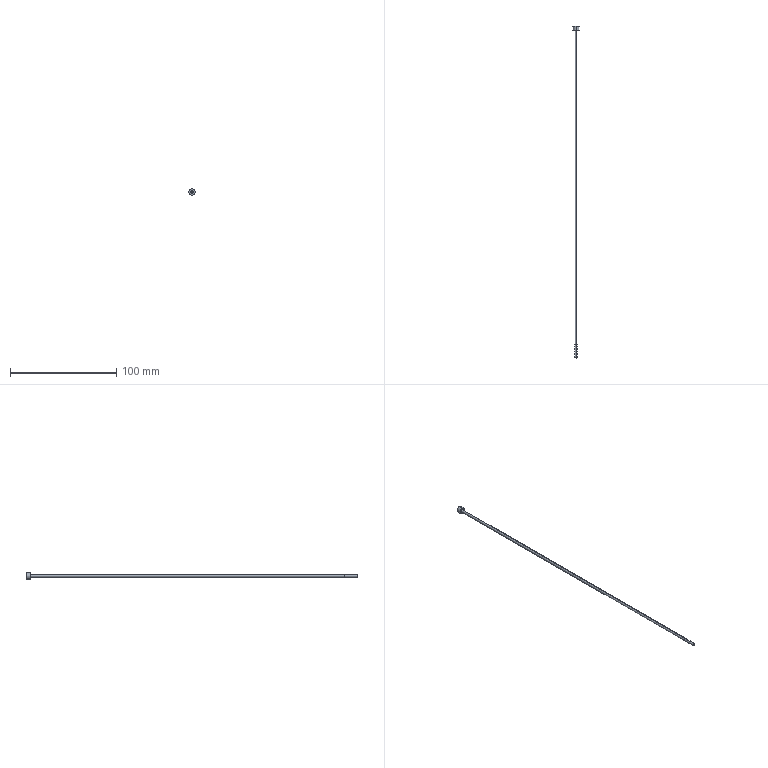Part | STEP file | 1 solid | 9 faces | box 6 x 312.335 x 6 mm | volume 1622 mm3 | cylinder 4 | plane 3 | cone 2 | commonest cylinder face diameters 2.5 x2 6 x2
STEP:
#1=CARTESIAN_POINT('',(0.,0.,0.));
#2=DIRECTION('',(0.,0.,1.));
#3=DIRECTION('',(1.,0.,0.));
#4=AXIS2_PLACEMENT_3D('',#1,#2,#3);
#5=CARTESIAN_POINT('',(-108.037,345.5,10.065));
#6=VERTEX_POINT('',#5);
#7=CARTESIAN_POINT('',(-108.037,345.5,16.065));
#8=VERTEX_POINT('',#7);
#9=CARTESIAN_POINT('',(-108.037,345.5,13.065));
#10=DIRECTION('',(0.,-1.,0.));
#11=DIRECTION('',(0.,0.,-1.));
#12=AXIS2_PLACEMENT_3D('',#9,#10,#11);
#13=CIRCLE('',#12,3.);
#14=CARTESIAN_POINT('',(-108.037,345.5,13.065));
#15=DIRECTION('',(0.,-1.,0.));
#16=DIRECTION('',(0.,0.,-1.));
#17=AXIS2_PLACEMENT_3D('',#14,#15,#16);
#18=CYLINDRICAL_SURFACE('',#17,3.);
#19=CARTESIAN_POINT('',(0.,0.));
#20=DIRECTION('',(1.,0.));
#21=VECTOR('',#20,1.);
#22=LINE('',#19,#21);
#23=(GEOMETRIC_REPRESENTATION_CONTEXT(2)PARAMETRIC_REPRESENTATION_CONTEXT()REPRESENTATION_CONTEXT('',''));
#24=DEFINITIONAL_REPRESENTATION('',(#22),#23);
#25=PCURVE('',#18,#24);
#26=CARTESIAN_POINT('',(-72.862,345.5,110.196));
#27=DIRECTION('',(0.,-1.,0.));
#28=DIRECTION('',(0.,0.,-1.));
#29=AXIS2_PLACEMENT_3D('',#26,#27,#28);
#30=PLANE('',#29);
#31=CARTESIAN_POINT('',(97.131,-35.175));
#32=DIRECTION('',(1.,0.));
#33=AXIS2_PLACEMENT_2D('',#31,#32);
#34=CIRCLE('',#33,3.);
#35=(GEOMETRIC_REPRESENTATION_CONTEXT(2)PARAMETRIC_REPRESENTATION_CONTEXT()REPRESENTATION_CONTEXT('',''));
#36=DEFINITIONAL_REPRESENTATION('',(#34),#35);
#37=PCURVE('',#30,#36);
#38=SURFACE_CURVE('',#13,(#25,#37),.PCURVE_S1.);
#39=EDGE_CURVE('',#6,#8,#38,.T.);
#40=ORIENTED_EDGE('',*,*,#39,.T.);
#41=CARTESIAN_POINT('',(-108.037,341.5,16.065));
#42=VERTEX_POINT('',#41);
#43=CARTESIAN_POINT('',(-108.037,345.5,16.065));
#44=DIRECTION('',(0.,-1.,0.));
#45=VECTOR('',#44,1.);
#46=LINE('',#43,#45);
#47=CARTESIAN_POINT('',(3.142,0.));
#48=DIRECTION('',(0.,1.));
#49=VECTOR('',#48,1.);
#50=LINE('',#47,#49);
#51=(GEOMETRIC_REPRESENTATION_CONTEXT(2)PARAMETRIC_REPRESENTATION_CONTEXT()REPRESENTATION_CONTEXT('',''));
#52=DEFINITIONAL_REPRESENTATION('',(#50),#51);
#53=PCURVE('',#18,#52);
#54=CARTESIAN_POINT('',(-108.037,345.5,13.065));
#55=DIRECTION('',(0.,-1.,0.));
#56=DIRECTION('',(0.,0.,-1.));
#57=AXIS2_PLACEMENT_3D('',#54,#55,#56);
#58=CYLINDRICAL_SURFACE('',#57,3.);
#59=CARTESIAN_POINT('',(3.142,0.));
#60=DIRECTION('',(0.,1.));
#61=VECTOR('',#60,1.);
#62=LINE('',#59,#61);
#63=(GEOMETRIC_REPRESENTATION_CONTEXT(2)PARAMETRIC_REPRESENTATION_CONTEXT()REPRESENTATION_CONTEXT('',''));
#64=DEFINITIONAL_REPRESENTATION('',(#62),#63);
#65=PCURVE('',#58,#64);
#66=SURFACE_CURVE('',#46,(#53,#65),.PCURVE_S1.);
#67=EDGE_CURVE('',#8,#42,#66,.T.);
#68=ORIENTED_EDGE('',*,*,#67,.T.);
#69=CARTESIAN_POINT('',(-108.037,341.5,10.065));
#70=VERTEX_POINT('',#69);
#71=CARTESIAN_POINT('',(-108.037,341.5,13.065));
#72=DIRECTION('',(0.,1.,0.));
#73=DIRECTION('',(0.,0.,1.));
#74=AXIS2_PLACEMENT_3D('',#71,#72,#73);
#75=CIRCLE('',#74,3.);
#76=CARTESIAN_POINT('',(3.142,4.));
#77=DIRECTION('',(-1.,0.));
#78=VECTOR('',#77,1.);
#79=LINE('',#76,#78);
#80=(GEOMETRIC_REPRESENTATION_CONTEXT(2)PARAMETRIC_REPRESENTATION_CONTEXT()REPRESENTATION_CONTEXT('',''));
#81=DEFINITIONAL_REPRESENTATION('',(#79),#80);
#82=PCURVE('',#18,#81);
#83=CARTESIAN_POINT('',(-108.037,341.5,13.065));
#84=DIRECTION('',(0.,-1.,0.));
#85=DIRECTION('',(0.,0.,-1.));
#86=AXIS2_PLACEMENT_3D('',#83,#84,#85);
#87=PLANE('',#86);
#88=CARTESIAN_POINT('',(-3.,0.));
#89=CARTESIAN_POINT('',(-3.,5.196));
#90=CARTESIAN_POINT('',(1.5,2.598));
#91=CARTESIAN_POINT('',(6.,0.));
#92=CARTESIAN_POINT('',(1.5,-2.598));
#93=CARTESIAN_POINT('',(-3.,-5.196));
#94=CARTESIAN_POINT('',(-3.,0.));
#95=(BOUNDED_CURVE()B_SPLINE_CURVE(2,(#88,#89,#90,#91,#92,#93,#94),.UNSPECIFIED.,.T.,.F.)B_SPLINE_CURVE_WITH_KNOTS((1,2,2,2,2,1),(-2.094,0.,2.094,4.189,6.283,8.378),.UNSPECIFIED.)CURVE()GEOMETRIC_REPRESENTATION_ITEM()RATIONAL_B_SPLINE_CURVE((1.,0.5,1.,0.5,1.,0.5,1.))REPRESENTATION_ITEM(''));
#96=(GEOMETRIC_REPRESENTATION_CONTEXT(2)PARAMETRIC_REPRESENTATION_CONTEXT()REPRESENTATION_CONTEXT('',''));
#97=DEFINITIONAL_REPRESENTATION('',(#95),#96);
#98=PCURVE('',#87,#97);
#99=SURFACE_CURVE('',#75,(#82,#98),.PCURVE_S1.);
#100=EDGE_CURVE('',#42,#70,#99,.T.);
#101=ORIENTED_EDGE('',*,*,#100,.T.);
#102=CARTESIAN_POINT('',(-108.037,345.5,10.065));
#103=DIRECTION('',(0.,-1.,0.));
#104=VECTOR('',#103,1.);
#105=LINE('',#102,#104);
#106=CARTESIAN_POINT('',(0.,0.));
#107=DIRECTION('',(0.,1.));
#108=VECTOR('',#107,1.);
#109=LINE('',#106,#108);
#110=(GEOMETRIC_REPRESENTATION_CONTEXT(2)PARAMETRIC_REPRESENTATION_CONTEXT()REPRESENTATION_CONTEXT('',''));
#111=DEFINITIONAL_REPRESENTATION('',(#109),#110);
#112=PCURVE('',#18,#111);
#113=CARTESIAN_POINT('',(6.283,0.));
#114=DIRECTION('',(0.,1.));
#115=VECTOR('',#114,1.);
#116=LINE('',#113,#115);
#117=(GEOMETRIC_REPRESENTATION_CONTEXT(2)PARAMETRIC_REPRESENTATION_CONTEXT()REPRESENTATION_CONTEXT('',''));
#118=DEFINITIONAL_REPRESENTATION('',(#116),#117);
#119=PCURVE('',#58,#118);
#120=SURFACE_CURVE('',#105,(#112,#119),.PCURVE_S1.);
#121=EDGE_CURVE('',#6,#70,#120,.T.);
#122=ORIENTED_EDGE('',*,*,#121,.F.);
#123=EDGE_LOOP('',(#40,#68,#101,#122));
#124=FACE_BOUND('',#123,.T.);
#125=ADVANCED_FACE('',(#124),#18,.T.);
#126=CARTESIAN_POINT('',(-108.037,33.165,14.207));
#127=VERTEX_POINT('',#126);
#128=CARTESIAN_POINT('',(-108.037,33.165,11.923));
#129=VERTEX_POINT('',#128);
#130=CARTESIAN_POINT('',(-108.037,33.165,13.065));
#131=DIRECTION('',(0.,1.,0.));
#132=DIRECTION('',(0.,0.,-1.));
#133=AXIS2_PLACEMENT_3D('',#130,#131,#132);
#134=CIRCLE('',#133,1.142);
#135=CARTESIAN_POINT('',(-108.037,46.23,13.065));
#136=DIRECTION('',(0.,1.,0.));
#137=DIRECTION('',(0.,0.,1.));
#138=AXIS2_PLACEMENT_3D('',#135,#136,#137);
#139=CONICAL_SURFACE('',#138,1.256,0.008727);
#140=CARTESIAN_POINT('',(-3.142,-13.065));
#141=DIRECTION('',(1.,0.));
#142=VECTOR('',#141,1.);
#143=LINE('',#140,#142);
#144=(GEOMETRIC_REPRESENTATION_CONTEXT(2)PARAMETRIC_REPRESENTATION_CONTEXT()REPRESENTATION_CONTEXT('',''));
#145=DEFINITIONAL_REPRESENTATION('',(#143),#144);
#146=PCURVE('',#139,#145);
#147=CARTESIAN_POINT('',(-108.037,33.165,13.065));
#148=DIRECTION('',(0.,-1.,0.));
#149=DIRECTION('',(0.,0.,-1.));
#150=AXIS2_PLACEMENT_3D('',#147,#148,#149);
#151=PLANE('',#150);
#152=CARTESIAN_POINT('',(1.142,0.));
#153=CARTESIAN_POINT('',(1.142,-1.978));
#154=CARTESIAN_POINT('',(-0.5711,-0.9892));
#155=CARTESIAN_POINT('',(-2.284,0.));
#156=CARTESIAN_POINT('',(-0.5711,0.9892));
#157=CARTESIAN_POINT('',(1.142,1.978));
#158=CARTESIAN_POINT('',(1.142,0.));
#159=(BOUNDED_CURVE()B_SPLINE_CURVE(2,(#152,#153,#154,#155,#156,#157,#158),.UNSPECIFIED.,.T.,.F.)B_SPLINE_CURVE_WITH_KNOTS((1,2,2,2,2,1),(-2.094,0.,2.094,4.189,6.283,8.378),.UNSPECIFIED.)CURVE()GEOMETRIC_REPRESENTATION_ITEM()RATIONAL_B_SPLINE_CURVE((1.,0.5,1.,0.5,1.,0.5,1.))REPRESENTATION_ITEM(''));
#160=(GEOMETRIC_REPRESENTATION_CONTEXT(2)PARAMETRIC_REPRESENTATION_CONTEXT()REPRESENTATION_CONTEXT('',''));
#161=DEFINITIONAL_REPRESENTATION('',(#159),#160);
#162=PCURVE('',#151,#161);
#163=SURFACE_CURVE('',#134,(#146,#162),.PCURVE_S1.);
#164=EDGE_CURVE('',#127,#129,#163,.T.);
#165=ORIENTED_EDGE('',*,*,#164,.T.);
#166=CARTESIAN_POINT('',(-108.037,45.514,11.815));
#167=VERTEX_POINT('',#166);
#168=CARTESIAN_POINT('',(-108.037,46.23,11.809));
#169=DIRECTION('',(0.,1.,-0.008727));
#170=VECTOR('',#169,1.);
#171=LINE('',#168,#170);
#172=CARTESIAN_POINT('',(3.142,0.));
#173=DIRECTION('',(0.,1.));
#174=VECTOR('',#173,1.);
#175=LINE('',#172,#174);
#176=(GEOMETRIC_REPRESENTATION_CONTEXT(2)PARAMETRIC_REPRESENTATION_CONTEXT()REPRESENTATION_CONTEXT('',''));
#177=DEFINITIONAL_REPRESENTATION('',(#175),#176);
#178=PCURVE('',#139,#177);
#179=CARTESIAN_POINT('',(-108.037,46.23,13.065));
#180=DIRECTION('',(0.,1.,0.));
#181=DIRECTION('',(0.,0.,1.));
#182=AXIS2_PLACEMENT_3D('',#179,#180,#181);
#183=CONICAL_SURFACE('',#182,1.256,0.008727);
#184=CARTESIAN_POINT('',(3.142,0.));
#185=DIRECTION('',(0.,1.));
#186=VECTOR('',#185,1.);
#187=LINE('',#184,#186);
#188=(GEOMETRIC_REPRESENTATION_CONTEXT(2)PARAMETRIC_REPRESENTATION_CONTEXT()REPRESENTATION_CONTEXT('',''));
#189=DEFINITIONAL_REPRESENTATION('',(#187),#188);
#190=PCURVE('',#183,#189);
#191=SURFACE_CURVE('',#171,(#178,#190),.PCURVE_S1.);
#192=EDGE_CURVE('',#129,#167,#191,.T.);
#193=ORIENTED_EDGE('',*,*,#192,.T.);
#194=CARTESIAN_POINT('',(-108.037,45.514,14.315));
#195=VERTEX_POINT('',#194);
#196=CARTESIAN_POINT('',(-108.037,45.514,13.065));
#197=DIRECTION('',(0.,1.,0.));
#198=DIRECTION('',(0.,0.,1.));
#199=AXIS2_PLACEMENT_3D('',#196,#197,#198);
#200=CIRCLE('',#199,1.25);
#201=CARTESIAN_POINT('',(0.,-0.7162));
#202=DIRECTION('',(1.,0.));
#203=VECTOR('',#202,1.);
#204=LINE('',#201,#203);
#205=(GEOMETRIC_REPRESENTATION_CONTEXT(2)PARAMETRIC_REPRESENTATION_CONTEXT()REPRESENTATION_CONTEXT('',''));
#206=DEFINITIONAL_REPRESENTATION('',(#204),#205);
#207=PCURVE('',#139,#206);
#208=CARTESIAN_POINT('',(-108.037,33.165,13.065));
#209=DIRECTION('',(0.,1.,0.));
#210=DIRECTION('',(0.,0.,1.));
#211=AXIS2_PLACEMENT_3D('',#208,#209,#210);
#212=CYLINDRICAL_SURFACE('',#211,1.25);
#213=CARTESIAN_POINT('',(0.,12.349));
#214=DIRECTION('',(1.,0.));
#215=VECTOR('',#214,1.);
#216=LINE('',#213,#215);
#217=(GEOMETRIC_REPRESENTATION_CONTEXT(2)PARAMETRIC_REPRESENTATION_CONTEXT()REPRESENTATION_CONTEXT('',''));
#218=DEFINITIONAL_REPRESENTATION('',(#216),#217);
#219=PCURVE('',#212,#218);
#220=SURFACE_CURVE('',#200,(#207,#219),.PCURVE_S1.);
#221=EDGE_CURVE('',#195,#167,#220,.T.);
#222=ORIENTED_EDGE('',*,*,#221,.F.);
#223=CARTESIAN_POINT('',(-108.037,46.23,14.321));
#224=DIRECTION('',(0.,1.,0.008727));
#225=VECTOR('',#224,1.);
#226=LINE('',#223,#225);
#227=CARTESIAN_POINT('',(0.,0.));
#228=DIRECTION('',(0.,1.));
#229=VECTOR('',#228,1.);
#230=LINE('',#227,#229);
#231=(GEOMETRIC_REPRESENTATION_CONTEXT(2)PARAMETRIC_REPRESENTATION_CONTEXT()REPRESENTATION_CONTEXT('',''));
#232=DEFINITIONAL_REPRESENTATION('',(#230),#231);
#233=PCURVE('',#139,#232);
#234=CARTESIAN_POINT('',(6.283,0.));
#235=DIRECTION('',(0.,1.));
#236=VECTOR('',#235,1.);
#237=LINE('',#234,#236);
#238=(GEOMETRIC_REPRESENTATION_CONTEXT(2)PARAMETRIC_REPRESENTATION_CONTEXT()REPRESENTATION_CONTEXT('',''));
#239=DEFINITIONAL_REPRESENTATION('',(#237),#238);
#240=PCURVE('',#183,#239);
#241=SURFACE_CURVE('',#226,(#233,#240),.PCURVE_S1.);
#242=EDGE_CURVE('',#127,#195,#241,.T.);
#243=ORIENTED_EDGE('',*,*,#242,.F.);
#244=EDGE_LOOP('',(#165,#193,#222,#243));
#245=FACE_BOUND('',#244,.T.);
#246=ADVANCED_FACE('',(#245),#139,.T.);
#247=ORIENTED_EDGE('',*,*,#221,.T.);
#248=CARTESIAN_POINT('',(-108.037,341.5,11.815));
#249=VERTEX_POINT('',#248);
#250=CARTESIAN_POINT('',(-108.037,33.165,11.815));
#251=DIRECTION('',(0.,1.,0.));
#252=VECTOR('',#251,1.);
#253=LINE('',#250,#252);
#254=CARTESIAN_POINT('',(3.142,0.));
#255=DIRECTION('',(0.,1.));
#256=VECTOR('',#255,1.);
#257=LINE('',#254,#256);
#258=(GEOMETRIC_REPRESENTATION_CONTEXT(2)PARAMETRIC_REPRESENTATION_CONTEXT()REPRESENTATION_CONTEXT('',''));
#259=DEFINITIONAL_REPRESENTATION('',(#257),#258);
#260=PCURVE('',#212,#259);
#261=CARTESIAN_POINT('',(-108.037,33.165,13.065));
#262=DIRECTION('',(0.,1.,0.));
#263=DIRECTION('',(0.,0.,1.));
#264=AXIS2_PLACEMENT_3D('',#261,#262,#263);
#265=CYLINDRICAL_SURFACE('',#264,1.25);
#266=CARTESIAN_POINT('',(3.142,0.));
#267=DIRECTION('',(0.,1.));
#268=VECTOR('',#267,1.);
#269=LINE('',#266,#268);
#270=(GEOMETRIC_REPRESENTATION_CONTEXT(2)PARAMETRIC_REPRESENTATION_CONTEXT()REPRESENTATION_CONTEXT('',''));
#271=DEFINITIONAL_REPRESENTATION('',(#269),#270);
#272=PCURVE('',#265,#271);
#273=SURFACE_CURVE('',#253,(#260,#272),.PCURVE_S1.);
#274=EDGE_CURVE('',#167,#249,#273,.T.);
#275=ORIENTED_EDGE('',*,*,#274,.T.);
#276=CARTESIAN_POINT('',(-108.037,341.5,14.315));
#277=VERTEX_POINT('',#276);
#278=CARTESIAN_POINT('',(-108.037,341.5,13.065));
#279=DIRECTION('',(0.,1.,0.));
#280=DIRECTION('',(0.,0.,-1.));
#281=AXIS2_PLACEMENT_3D('',#278,#279,#280);
#282=CIRCLE('',#281,1.25);
#283=CARTESIAN_POINT('',(-3.142,308.335));
#284=DIRECTION('',(1.,0.));
#285=VECTOR('',#284,1.);
#286=LINE('',#283,#285);
#287=(GEOMETRIC_REPRESENTATION_CONTEXT(2)PARAMETRIC_REPRESENTATION_CONTEXT()REPRESENTATION_CONTEXT('',''));
#288=DEFINITIONAL_REPRESENTATION('',(#286),#287);
#289=PCURVE('',#212,#288);
#290=CARTESIAN_POINT('',(1.25,0.));
#291=CARTESIAN_POINT('',(1.25,-2.165));
#292=CARTESIAN_POINT('',(-0.625,-1.083));
#293=CARTESIAN_POINT('',(-2.5,0.));
#294=CARTESIAN_POINT('',(-0.625,1.083));
#295=CARTESIAN_POINT('',(1.25,2.165));
#296=CARTESIAN_POINT('',(1.25,0.));
#297=(BOUNDED_CURVE()B_SPLINE_CURVE(2,(#290,#291,#292,#293,#294,#295,#296),.UNSPECIFIED.,.T.,.F.)B_SPLINE_CURVE_WITH_KNOTS((1,2,2,2,2,1),(-2.094,0.,2.094,4.189,6.283,8.378),.UNSPECIFIED.)CURVE()GEOMETRIC_REPRESENTATION_ITEM()RATIONAL_B_SPLINE_CURVE((1.,0.5,1.,0.5,1.,0.5,1.))REPRESENTATION_ITEM(''));
#298=(GEOMETRIC_REPRESENTATION_CONTEXT(2)PARAMETRIC_REPRESENTATION_CONTEXT()REPRESENTATION_CONTEXT('',''));
#299=DEFINITIONAL_REPRESENTATION('',(#297),#298);
#300=PCURVE('',#87,#299);
#301=SURFACE_CURVE('',#282,(#289,#300),.PCURVE_S1.);
#302=EDGE_CURVE('',#277,#249,#301,.T.);
#303=ORIENTED_EDGE('',*,*,#302,.F.);
#304=CARTESIAN_POINT('',(-108.037,33.165,14.315));
#305=DIRECTION('',(0.,1.,0.));
#306=VECTOR('',#305,1.);
#307=LINE('',#304,#306);
#308=CARTESIAN_POINT('',(0.,0.));
#309=DIRECTION('',(0.,1.));
#310=VECTOR('',#309,1.);
#311=LINE('',#308,#310);
#312=(GEOMETRIC_REPRESENTATION_CONTEXT(2)PARAMETRIC_REPRESENTATION_CONTEXT()REPRESENTATION_CONTEXT('',''));
#313=DEFINITIONAL_REPRESENTATION('',(#311),#312);
#314=PCURVE('',#212,#313);
#315=CARTESIAN_POINT('',(6.283,0.));
#316=DIRECTION('',(0.,1.));
#317=VECTOR('',#316,1.);
#318=LINE('',#315,#317);
#319=(GEOMETRIC_REPRESENTATION_CONTEXT(2)PARAMETRIC_REPRESENTATION_CONTEXT()REPRESENTATION_CONTEXT('',''));
#320=DEFINITIONAL_REPRESENTATION('',(#318),#319);
#321=PCURVE('',#265,#320);
#322=SURFACE_CURVE('',#307,(#314,#321),.PCURVE_S1.);
#323=EDGE_CURVE('',#195,#277,#322,.T.);
#324=ORIENTED_EDGE('',*,*,#323,.F.);
#325=EDGE_LOOP('',(#247,#275,#303,#324));
#326=FACE_BOUND('',#325,.T.);
#327=ADVANCED_FACE('',(#326),#212,.T.);
#328=ORIENTED_EDGE('',*,*,#274,.F.);
#329=CARTESIAN_POINT('',(-108.037,45.514,13.065));
#330=DIRECTION('',(0.,1.,0.));
#331=DIRECTION('',(0.,0.,1.));
#332=AXIS2_PLACEMENT_3D('',#329,#330,#331);
#333=CIRCLE('',#332,1.25);
#334=CARTESIAN_POINT('',(0.,12.349));
#335=DIRECTION('',(1.,0.));
#336=VECTOR('',#335,1.);
#337=LINE('',#334,#336);
#338=(GEOMETRIC_REPRESENTATION_CONTEXT(2)PARAMETRIC_REPRESENTATION_CONTEXT()REPRESENTATION_CONTEXT('',''));
#339=DEFINITIONAL_REPRESENTATION('',(#337),#338);
#340=PCURVE('',#265,#339);
#341=CARTESIAN_POINT('',(0.,-0.7162));
#342=DIRECTION('',(1.,0.));
#343=VECTOR('',#342,1.);
#344=LINE('',#341,#343);
#345=(GEOMETRIC_REPRESENTATION_CONTEXT(2)PARAMETRIC_REPRESENTATION_CONTEXT()REPRESENTATION_CONTEXT('',''));
#346=DEFINITIONAL_REPRESENTATION('',(#344),#345);
#347=PCURVE('',#183,#346);
#348=SURFACE_CURVE('',#333,(#340,#347),.PCURVE_S1.);
#349=EDGE_CURVE('',#167,#195,#348,.T.);
#350=ORIENTED_EDGE('',*,*,#349,.T.);
#351=ORIENTED_EDGE('',*,*,#323,.T.);
#352=CARTESIAN_POINT('',(-108.037,341.5,13.065));
#353=DIRECTION('',(0.,1.,0.));
#354=DIRECTION('',(0.,0.,-1.));
#355=AXIS2_PLACEMENT_3D('',#352,#353,#354);
#356=CIRCLE('',#355,1.25);
#357=CARTESIAN_POINT('',(3.142,308.335));
#358=DIRECTION('',(1.,0.));
#359=VECTOR('',#358,1.);
#360=LINE('',#357,#359);
#361=(GEOMETRIC_REPRESENTATION_CONTEXT(2)PARAMETRIC_REPRESENTATION_CONTEXT()REPRESENTATION_CONTEXT('',''));
#362=DEFINITIONAL_REPRESENTATION('',(#360),#361);
#363=PCURVE('',#265,#362);
#364=CARTESIAN_POINT('',(1.25,0.));
#365=CARTESIAN_POINT('',(1.25,-2.165));
#366=CARTESIAN_POINT('',(-0.625,-1.083));
#367=CARTESIAN_POINT('',(-2.5,0.));
#368=CARTESIAN_POINT('',(-0.625,1.083));
#369=CARTESIAN_POINT('',(1.25,2.165));
#370=CARTESIAN_POINT('',(1.25,0.));
#371=(BOUNDED_CURVE()B_SPLINE_CURVE(2,(#364,#365,#366,#367,#368,#369,#370),.UNSPECIFIED.,.T.,.F.)B_SPLINE_CURVE_WITH_KNOTS((1,2,2,2,2,1),(-2.094,0.,2.094,4.189,6.283,8.378),.UNSPECIFIED.)CURVE()GEOMETRIC_REPRESENTATION_ITEM()RATIONAL_B_SPLINE_CURVE((1.,0.5,1.,0.5,1.,0.5,1.))REPRESENTATION_ITEM(''));
#372=(GEOMETRIC_REPRESENTATION_CONTEXT(2)PARAMETRIC_REPRESENTATION_CONTEXT()REPRESENTATION_CONTEXT('',''));
#373=DEFINITIONAL_REPRESENTATION('',(#371),#372);
#374=PCURVE('',#87,#373);
#375=SURFACE_CURVE('',#356,(#363,#374),.PCURVE_S1.);
#376=EDGE_CURVE('',#249,#277,#375,.T.);
#377=ORIENTED_EDGE('',*,*,#376,.F.);
#378=EDGE_LOOP('',(#328,#350,#351,#377));
#379=FACE_BOUND('',#378,.T.);
#380=ADVANCED_FACE('',(#379),#265,.T.);
#381=ORIENTED_EDGE('',*,*,#192,.F.);
#382=CARTESIAN_POINT('',(-108.037,33.165,13.065));
#383=DIRECTION('',(0.,1.,0.));
#384=DIRECTION('',(0.,0.,-1.));
#385=AXIS2_PLACEMENT_3D('',#382,#383,#384);
#386=CIRCLE('',#385,1.142);
#387=CARTESIAN_POINT('',(3.142,-13.065));
#388=DIRECTION('',(1.,0.));
#389=VECTOR('',#388,1.);
#390=LINE('',#387,#389);
#391=(GEOMETRIC_REPRESENTATION_CONTEXT(2)PARAMETRIC_REPRESENTATION_CONTEXT()REPRESENTATION_CONTEXT('',''));
#392=DEFINITIONAL_REPRESENTATION('',(#390),#391);
#393=PCURVE('',#183,#392);
#394=CARTESIAN_POINT('',(1.142,0.));
#395=CARTESIAN_POINT('',(1.142,-1.978));
#396=CARTESIAN_POINT('',(-0.5711,-0.9892));
#397=CARTESIAN_POINT('',(-2.284,0.));
#398=CARTESIAN_POINT('',(-0.5711,0.9892));
#399=CARTESIAN_POINT('',(1.142,1.978));
#400=CARTESIAN_POINT('',(1.142,0.));
#401=(BOUNDED_CURVE()B_SPLINE_CURVE(2,(#394,#395,#396,#397,#398,#399,#400),.UNSPECIFIED.,.T.,.F.)B_SPLINE_CURVE_WITH_KNOTS((1,2,2,2,2,1),(-2.094,0.,2.094,4.189,6.283,8.378),.UNSPECIFIED.)CURVE()GEOMETRIC_REPRESENTATION_ITEM()RATIONAL_B_SPLINE_CURVE((1.,0.5,1.,0.5,1.,0.5,1.))REPRESENTATION_ITEM(''));
#402=(GEOMETRIC_REPRESENTATION_CONTEXT(2)PARAMETRIC_REPRESENTATION_CONTEXT()REPRESENTATION_CONTEXT('',''));
#403=DEFINITIONAL_REPRESENTATION('',(#401),#402);
#404=PCURVE('',#151,#403);
#405=SURFACE_CURVE('',#386,(#393,#404),.PCURVE_S1.);
#406=EDGE_CURVE('',#129,#127,#405,.T.);
#407=ORIENTED_EDGE('',*,*,#406,.T.);
#408=ORIENTED_EDGE('',*,*,#242,.T.);
#409=ORIENTED_EDGE('',*,*,#349,.F.);
#410=EDGE_LOOP('',(#381,#407,#408,#409));
#411=FACE_BOUND('',#410,.T.);
#412=ADVANCED_FACE('',(#411),#183,.T.);
#413=ORIENTED_EDGE('',*,*,#164,.F.);
#414=ORIENTED_EDGE('',*,*,#406,.F.);
#415=EDGE_LOOP('',(#413,#414));
#416=FACE_BOUND('',#415,.T.);
#417=ADVANCED_FACE('',(#416),#151,.T.);
#418=ORIENTED_EDGE('',*,*,#302,.T.);
#419=ORIENTED_EDGE('',*,*,#376,.T.);
#420=EDGE_LOOP('',(#418,#419));
#421=FACE_BOUND('',#420,.T.);
#422=CARTESIAN_POINT('',(-108.037,341.5,13.065));
#423=DIRECTION('',(0.,1.,0.));
#424=DIRECTION('',(0.,0.,1.));
#425=AXIS2_PLACEMENT_3D('',#422,#423,#424);
#426=CIRCLE('',#425,3.);
#427=CARTESIAN_POINT('',(-3.,0.));
#428=CARTESIAN_POINT('',(-3.,5.196));
#429=CARTESIAN_POINT('',(1.5,2.598));
#430=CARTESIAN_POINT('',(6.,0.));
#431=CARTESIAN_POINT('',(1.5,-2.598));
#432=CARTESIAN_POINT('',(-3.,-5.196));
#433=CARTESIAN_POINT('',(-3.,0.));
#434=(BOUNDED_CURVE()B_SPLINE_CURVE(2,(#427,#428,#429,#430,#431,#432,#433),.UNSPECIFIED.,.T.,.F.)B_SPLINE_CURVE_WITH_KNOTS((1,2,2,2,2,1),(-2.094,0.,2.094,4.189,6.283,8.378),.UNSPECIFIED.)CURVE()GEOMETRIC_REPRESENTATION_ITEM()RATIONAL_B_SPLINE_CURVE((1.,0.5,1.,0.5,1.,0.5,1.))REPRESENTATION_ITEM(''));
#435=(GEOMETRIC_REPRESENTATION_CONTEXT(2)PARAMETRIC_REPRESENTATION_CONTEXT()REPRESENTATION_CONTEXT('',''));
#436=DEFINITIONAL_REPRESENTATION('',(#434),#435);
#437=PCURVE('',#87,#436);
#438=CARTESIAN_POINT('',(9.425,4.));
#439=DIRECTION('',(-1.,0.));
#440=VECTOR('',#439,1.);
#441=LINE('',#438,#440);
#442=(GEOMETRIC_REPRESENTATION_CONTEXT(2)PARAMETRIC_REPRESENTATION_CONTEXT()REPRESENTATION_CONTEXT('',''));
#443=DEFINITIONAL_REPRESENTATION('',(#441),#442);
#444=PCURVE('',#58,#443);
#445=SURFACE_CURVE('',#426,(#437,#444),.PCURVE_S1.);
#446=EDGE_CURVE('',#70,#42,#445,.T.);
#447=ORIENTED_EDGE('',*,*,#446,.F.);
#448=ORIENTED_EDGE('',*,*,#100,.F.);
#449=EDGE_LOOP('',(#447,#448));
#450=FACE_BOUND('',#449,.T.);
#451=ADVANCED_FACE('',(#421,#450),#87,.T.);
#452=ORIENTED_EDGE('',*,*,#67,.F.);
#453=CARTESIAN_POINT('',(-108.037,345.5,13.065));
#454=DIRECTION('',(0.,-1.,0.));
#455=DIRECTION('',(0.,0.,-1.));
#456=AXIS2_PLACEMENT_3D('',#453,#454,#455);
#457=CIRCLE('',#456,3.);
#458=CARTESIAN_POINT('',(0.,0.));
#459=DIRECTION('',(1.,0.));
#460=VECTOR('',#459,1.);
#461=LINE('',#458,#460);
#462=(GEOMETRIC_REPRESENTATION_CONTEXT(2)PARAMETRIC_REPRESENTATION_CONTEXT()REPRESENTATION_CONTEXT('',''));
#463=DEFINITIONAL_REPRESENTATION('',(#461),#462);
#464=PCURVE('',#58,#463);
#465=CARTESIAN_POINT('',(97.131,-35.175));
#466=DIRECTION('',(1.,0.));
#467=AXIS2_PLACEMENT_2D('',#465,#466);
#468=CIRCLE('',#467,3.);
#469=(GEOMETRIC_REPRESENTATION_CONTEXT(2)PARAMETRIC_REPRESENTATION_CONTEXT()REPRESENTATION_CONTEXT('',''));
#470=DEFINITIONAL_REPRESENTATION('',(#468),#469);
#471=PCURVE('',#30,#470);
#472=SURFACE_CURVE('',#457,(#464,#471),.PCURVE_S1.);
#473=EDGE_CURVE('',#8,#6,#472,.T.);
#474=ORIENTED_EDGE('',*,*,#473,.T.);
#475=ORIENTED_EDGE('',*,*,#121,.T.);
#476=ORIENTED_EDGE('',*,*,#446,.T.);
#477=EDGE_LOOP('',(#452,#474,#475,#476));
#478=FACE_BOUND('',#477,.T.);
#479=ADVANCED_FACE('',(#478),#58,.T.);
#480=ORIENTED_EDGE('',*,*,#39,.F.);
#481=ORIENTED_EDGE('',*,*,#473,.F.);
#482=EDGE_LOOP('',(#480,#481));
#483=FACE_BOUND('',#482,.T.);
#484=ADVANCED_FACE('',(#483),#30,.F.);
#485=CLOSED_SHELL('',(#125,#246,#327,#380,#412,#417,#451,#479,#484));
#486=MANIFOLD_SOLID_BREP('',#485);
#487=(LENGTH_UNIT()NAMED_UNIT(*)SI_UNIT(.MILLI.,.METRE.));
#488=UNCERTAINTY_MEASURE_WITH_UNIT(LENGTH_MEASURE(0.0000001),#487,'','');
#489=(NAMED_UNIT(*)PLANE_ANGLE_UNIT()SI_UNIT($,.RADIAN.));
#490=(NAMED_UNIT(*)SI_UNIT($,.STERADIAN.)SOLID_ANGLE_UNIT());
#491=(GEOMETRIC_REPRESENTATION_CONTEXT(3)GLOBAL_UNCERTAINTY_ASSIGNED_CONTEXT((#488))GLOBAL_UNIT_ASSIGNED_CONTEXT((#487,#489,#490))REPRESENTATION_CONTEXT('',''));
#492=ADVANCED_BREP_SHAPE_REPRESENTATION('',(#4,#486),#491);